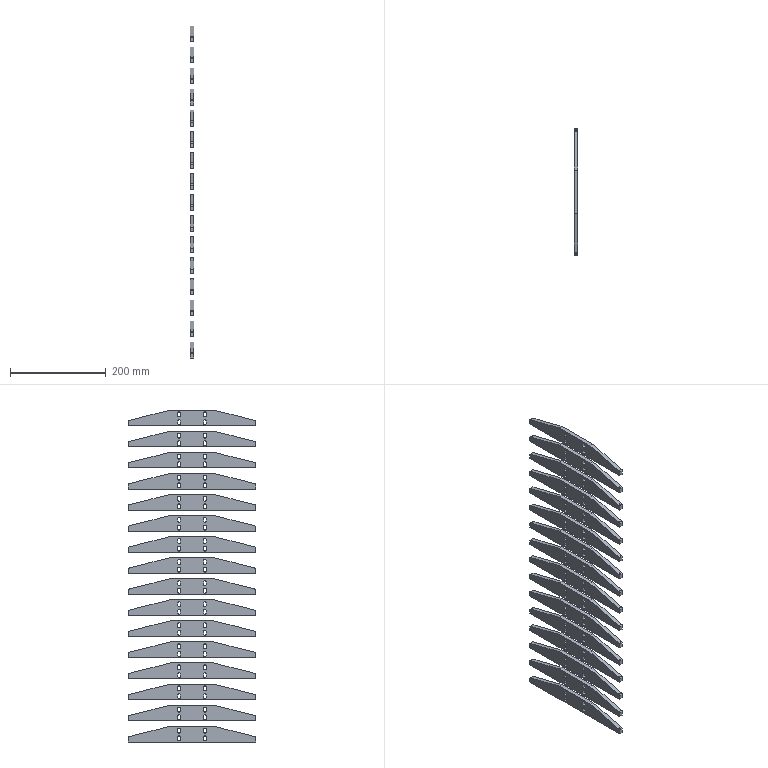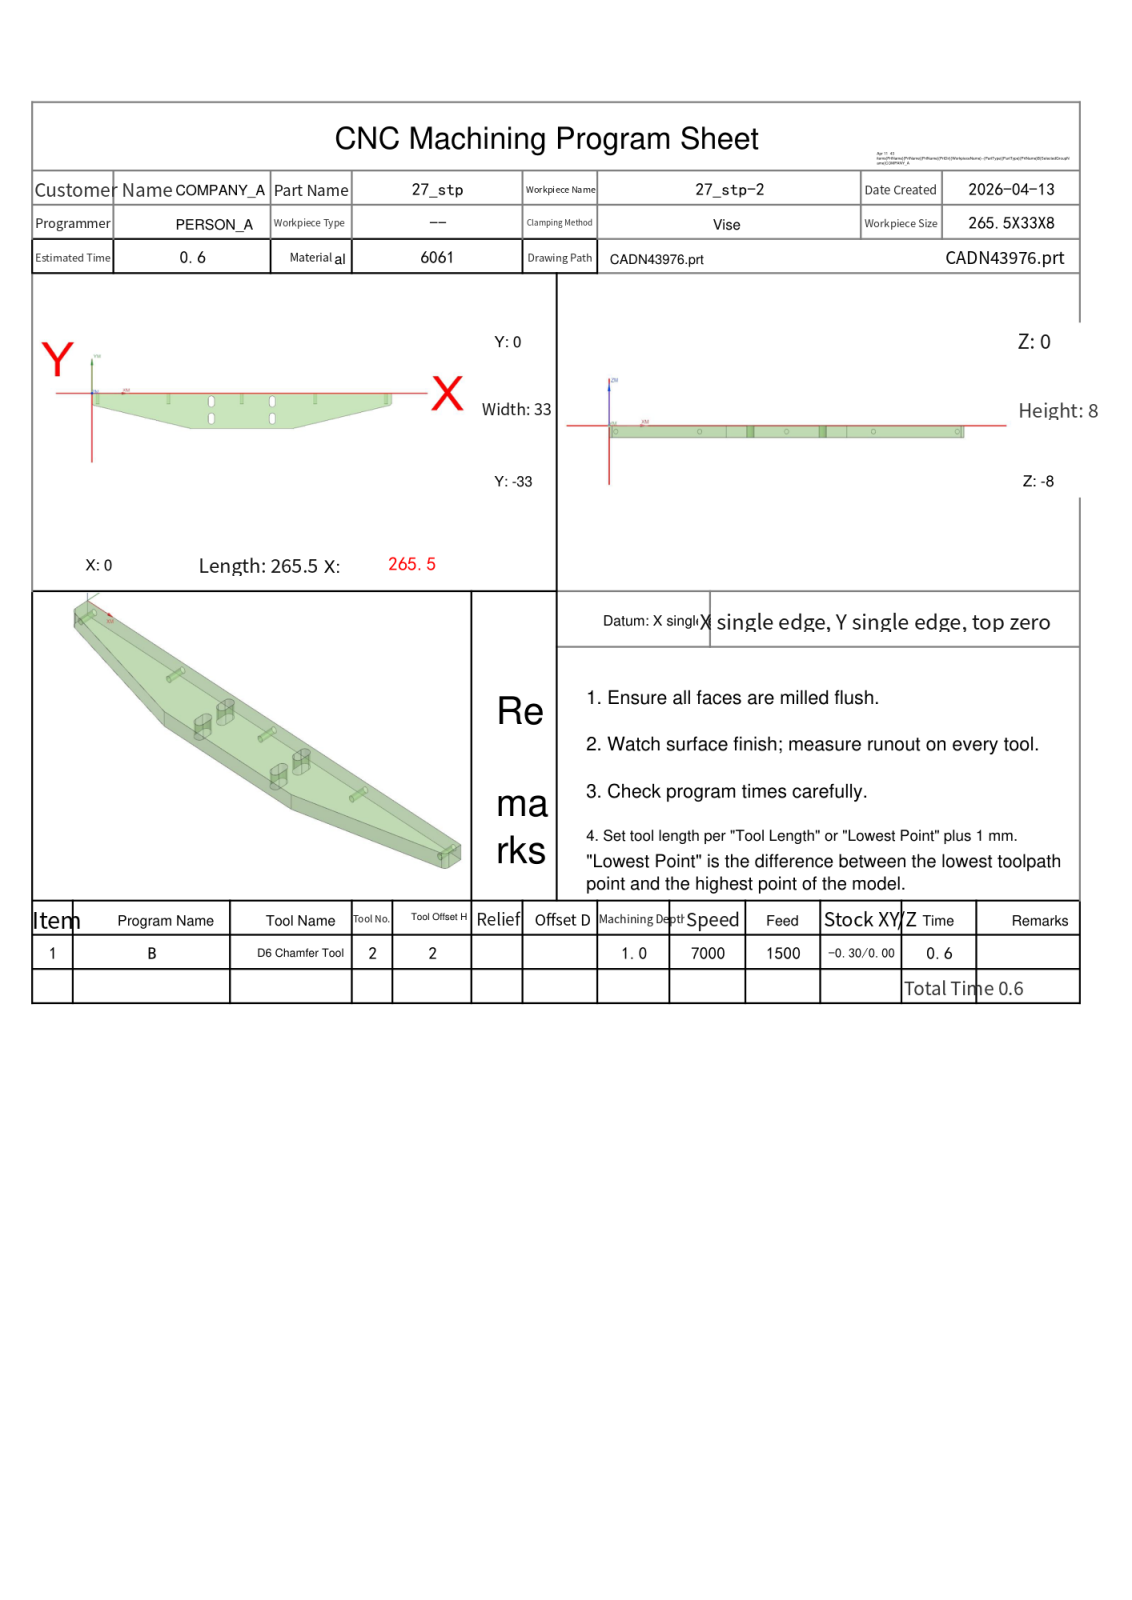NC program | NX | posted by the shop | part box 8 x 265.5 x 693 mm
Whole program:
%
O0001
(Machine time: 0.74 MIN)
(===Total Tool:1===)
(T2=D6 Chamfer Tool   D=6.   R=0.   D-  H02 Z=-1.   )
G80 G90 G17 G49 G40
G91 G28 Z0
M01
N1 T02 M06
(D6 Chamfer Tool  D=6. R=0. H=02 ce=-0.30 di=0.00)
G00 G90 G54 X161.038 Y-19.607 M03 S7000
G43 H02 Z50.
M08
Z2.5
G01 X160.975 Y-19.552 Z2.47 F1500.
X160.721 Y-19.391 Z2.361
X160.447 Y-19.269 Z2.251
X160.159 Y-19.188 Z2.142
X159.861 Y-19.15 Z2.033
X159.639 Z1.952
X159.341 Y-19.188 Z1.843
X159.053 Y-19.269 Z1.734
X158.779 Y-19.391 Z1.625
X158.525 Y-19.552 Z1.515
X158.298 Y-19.748 Z1.406
X158.102 Y-19.975 Z1.297
X157.941 Y-20.229 Z1.188
X157.819 Y-20.503 Z1.079
X157.738 Y-20.791 Z.969
X157.7 Y-21.089 Z.86
Y-26.2 Z-1.
G03 X159.75 Y-28.25 I2.05 J0.0
X161.8 Y-26.2 I0.0 J2.05
G01 Y-21.2
G03 X159.75 Y-19.15 I-2.05 J0.0
X157.7 Y-21.2 I0.0 J-2.05
G01 Y-26.2
G03 X157.761 Y-26.695 I2.05 J0.0
G01 Z1.5
G00 Z50.
X161.038 Y-3.607
Z2.5
G01 X160.975 Y-3.552 Z2.47
X160.721 Y-3.391 Z2.361
X160.447 Y-3.269 Z2.251
X160.159 Y-3.188 Z2.142
X159.861 Y-3.15 Z2.033
X159.639 Z1.952
X159.341 Y-3.188 Z1.843
X159.053 Y-3.269 Z1.734
X158.779 Y-3.391 Z1.625
X158.525 Y-3.552 Z1.515
X158.298 Y-3.748 Z1.406
X158.102 Y-3.975 Z1.297
X157.941 Y-4.229 Z1.188
X157.819 Y-4.503 Z1.079
X157.738 Y-4.791 Z.969
X157.7 Y-5.089 Z.86
Y-10.2 Z-1.
G03 X159.75 Y-12.25 I2.05 J0.0
X161.8 Y-10.2 I0.0 J2.05
G01 Y-5.2
G03 X159.75 Y-3.15 I-2.05 J0.0
X157.7 Y-5.2 I0.0 J-2.05
G01 Y-10.2
G03 X157.761 Y-10.695 I2.05 J0.0
G01 Z1.5
G00 Z50.
X-.7 Y-8.343
Z2.5
G01 Y-.222 Z-.456
X-.664 Y-.023 Z-.529
X-.589 Y.165 Z-.603
X-.477 Y.334 Z-.677
X-.334 Y.477 Z-.751
X-.165 Y.589 Z-.824
X.023 Y.664 Z-.898
X.222 Y.7 Z-.972
X.3 Z-1.
X265.2
G02 X266.2 Y-.3 I0.0 J-1.
G01 Y-8.512
G02 X263.407 Y-12.099 I-3.7 J0.0
G01 X178.123 Y-33.669
G02 X177.878 Y-33.7 I-.245 J.969
G01 X87.622
G02 X87.377 Y-33.669 I0.0 J1.
G01 X2.093 Y-12.099
G02 X-.7 Y-8.512 I.907 J3.587
G01 Y-.3
G02 X.3 Y.7 I1. J0.0
G01 X.8
Z1.5
G00 Z50.
X107.038 Y-3.607
Z2.5
G01 X106.975 Y-3.552 Z2.47
X106.721 Y-3.391 Z2.361
X106.447 Y-3.269 Z2.251
X106.159 Y-3.188 Z2.142
X105.861 Y-3.15 Z2.033
X105.639 Z1.952
X105.341 Y-3.188 Z1.843
X105.053 Y-3.269 Z1.734
X104.779 Y-3.391 Z1.625
X104.525 Y-3.552 Z1.515
X104.298 Y-3.748 Z1.406
X104.102 Y-3.975 Z1.297
X103.941 Y-4.229 Z1.188
X103.819 Y-4.503 Z1.079
X103.738 Y-4.791 Z.969
X103.7 Y-5.089 Z.86
Y-10.2 Z-1.
G03 X105.75 Y-12.25 I2.05 J0.0
X107.8 Y-10.2 I0.0 J2.05
G01 Y-5.2
G03 X105.75 Y-3.15 I-2.05 J0.0
X103.7 Y-5.2 I0.0 J-2.05
G01 Y-10.2
G03 X103.761 Y-10.695 I2.05 J0.0
G01 Z1.5
G00 Z50.
X107.038 Y-19.607
Z2.5
G01 X106.975 Y-19.552 Z2.47
X106.721 Y-19.391 Z2.361
X106.447 Y-19.269 Z2.251
X106.159 Y-19.188 Z2.142
X105.861 Y-19.15 Z2.033
X105.639 Z1.952
X105.341 Y-19.188 Z1.843
X105.053 Y-19.269 Z1.734
X104.779 Y-19.391 Z1.625
X104.525 Y-19.552 Z1.515
X104.298 Y-19.748 Z1.406
X104.102 Y-19.975 Z1.297
X103.941 Y-20.229 Z1.188
X103.819 Y-20.503 Z1.079
X103.738 Y-20.791 Z.969
X103.7 Y-21.089 Z.86
Y-26.2 Z-1.
G03 X105.75 Y-28.25 I2.05 J0.0
X107.8 Y-26.2 I0.0 J2.05
G01 Y-21.2
G03 X105.75 Y-19.15 I-2.05 J0.0
X103.7 Y-21.2 I0.0 J-2.05
G01 Y-26.2
G03 X103.761 Y-26.695 I2.05 J0.0
G01 Z1.5
G00 Z50.
M05
M09
G91 G28 Z0.0
G91 G28 Y0.0
M30
%